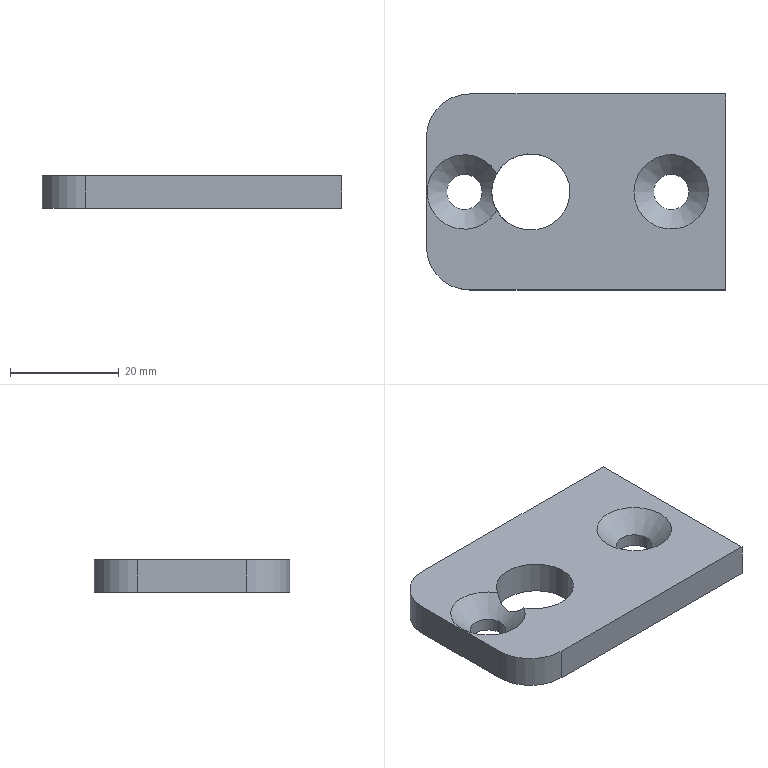Part | STEP file | solid 58 | 1 solid | 13 faces | box 55 x 36 x 6 mm | volume 10013 mm3 | plane 6 | cylinder 4 | cone 2 | other 1 | commonest cylinder face diameters 6.5 x2 16 x2